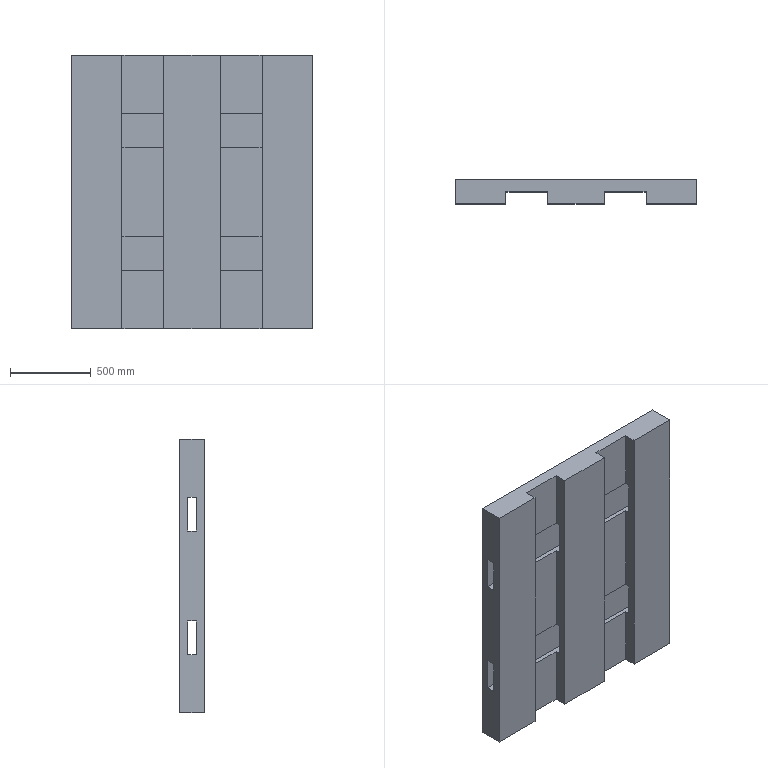Part | STEP file | Tray | 1 solid | 30 faces | box 1500 x 150 x 1700 mm | volume 287460631 mm3 | plane 30
STEP:
#1=CARTESIAN_POINT('',(-750.,-75.,0.));
#2=VERTEX_POINT('',#1);
#3=CARTESIAN_POINT('',(-435.,-75.,0.));
#4=VERTEX_POINT('',#3);
#5=CARTESIAN_POINT('',(-750.,-75.,0.));
#6=DIRECTION('',(1.,0.,0.));
#7=VECTOR('',#6,1000.);
#8=LINE('',#5,#7);
#9=EDGE_CURVE('',#2,#4,#8,.T.);
#10=ORIENTED_EDGE('',*,*,#9,.T.);
#11=CARTESIAN_POINT('',(-435.,-75.,1700.));
#12=VERTEX_POINT('',#11);
#13=CARTESIAN_POINT('',(-435.,-75.,-300.));
#14=DIRECTION('',(0.,0.,1.));
#15=VECTOR('',#14,1000.);
#16=LINE('',#13,#15);
#17=EDGE_CURVE('',#4,#12,#16,.T.);
#18=ORIENTED_EDGE('',*,*,#17,.T.);
#19=CARTESIAN_POINT('',(-750.,-75.,1700.));
#20=VERTEX_POINT('',#19);
#21=CARTESIAN_POINT('',(-750.,-75.,1700.));
#22=DIRECTION('',(1.,0.,0.));
#23=VECTOR('',#22,1000.);
#24=LINE('',#21,#23);
#25=EDGE_CURVE('',#20,#12,#24,.T.);
#26=ORIENTED_EDGE('',*,*,#25,.F.);
#27=CARTESIAN_POINT('',(-750.,-75.,1700.));
#28=DIRECTION('',(0.,0.,-1.));
#29=VECTOR('',#28,1000.);
#30=LINE('',#27,#29);
#31=EDGE_CURVE('',#20,#2,#30,.T.);
#32=ORIENTED_EDGE('',*,*,#31,.T.);
#33=EDGE_LOOP('',(#10,#18,#26,#32));
#34=FACE_OUTER_BOUND('',#33,.T.);
#35=CARTESIAN_POINT('',(-750.,-75.,1700.));
#36=DIRECTION('',(0.,1.,0.));
#37=DIRECTION('',(0.,0.,1.));
#38=AXIS2_PLACEMENT_3D('',#35,#36,#37);
#39=PLANE('',#38);
#40=ADVANCED_FACE('',(#34),#39,.F.);
#41=CARTESIAN_POINT('',(435.,-75.,1700.));
#42=VERTEX_POINT('',#41);
#43=CARTESIAN_POINT('',(750.,-75.,1700.));
#44=VERTEX_POINT('',#43);
#45=CARTESIAN_POINT('',(-750.,-75.,1700.));
#46=DIRECTION('',(1.,0.,0.));
#47=VECTOR('',#46,1000.);
#48=LINE('',#45,#47);
#49=EDGE_CURVE('',#42,#44,#48,.T.);
#50=ORIENTED_EDGE('',*,*,#49,.F.);
#51=CARTESIAN_POINT('',(435.,-75.,0.));
#52=VERTEX_POINT('',#51);
#53=CARTESIAN_POINT('',(435.,-75.,-300.));
#54=DIRECTION('',(0.,0.,1.));
#55=VECTOR('',#54,1000.);
#56=LINE('',#53,#55);
#57=EDGE_CURVE('',#52,#42,#56,.T.);
#58=ORIENTED_EDGE('',*,*,#57,.F.);
#59=CARTESIAN_POINT('',(750.,-75.,0.));
#60=VERTEX_POINT('',#59);
#61=CARTESIAN_POINT('',(-750.,-75.,0.));
#62=DIRECTION('',(1.,0.,0.));
#63=VECTOR('',#62,1000.);
#64=LINE('',#61,#63);
#65=EDGE_CURVE('',#52,#60,#64,.T.);
#66=ORIENTED_EDGE('',*,*,#65,.T.);
#67=CARTESIAN_POINT('',(750.,-75.,1700.));
#68=DIRECTION('',(0.,0.,-1.));
#69=VECTOR('',#68,1000.);
#70=LINE('',#67,#69);
#71=EDGE_CURVE('',#44,#60,#70,.T.);
#72=ORIENTED_EDGE('',*,*,#71,.F.);
#73=EDGE_LOOP('',(#50,#58,#66,#72));
#74=FACE_OUTER_BOUND('',#73,.T.);
#75=CARTESIAN_POINT('',(-750.,-75.,1700.));
#76=DIRECTION('',(0.,1.,0.));
#77=DIRECTION('',(0.,0.,1.));
#78=AXIS2_PLACEMENT_3D('',#75,#76,#77);
#79=PLANE('',#78);
#80=ADVANCED_FACE('',(#74),#79,.F.);
#81=CARTESIAN_POINT('',(-435.,-27.67,1338.848));
#82=VERTEX_POINT('',#81);
#83=CARTESIAN_POINT('',(-750.,-27.67,1338.848));
#84=VERTEX_POINT('',#83);
#85=CARTESIAN_POINT('',(1508.,-27.67,1338.848));
#86=DIRECTION('',(-1.,0.,0.));
#87=VECTOR('',#86,1000.);
#88=LINE('',#85,#87);
#89=EDGE_CURVE('',#82,#84,#88,.T.);
#90=ORIENTED_EDGE('',*,*,#89,.F.);
#91=CARTESIAN_POINT('',(-435.,-27.67,1129.441));
#92=VERTEX_POINT('',#91);
#93=CARTESIAN_POINT('',(-435.,-27.67,1338.848));
#94=DIRECTION('',(0.,0.,-1.));
#95=VECTOR('',#94,1000.);
#96=LINE('',#93,#95);
#97=EDGE_CURVE('',#82,#92,#96,.T.);
#98=ORIENTED_EDGE('',*,*,#97,.T.);
#99=CARTESIAN_POINT('',(-750.,-27.67,1129.441));
#100=VERTEX_POINT('',#99);
#101=CARTESIAN_POINT('',(1508.,-27.67,1129.441));
#102=DIRECTION('',(-1.,0.,0.));
#103=VECTOR('',#102,1000.);
#104=LINE('',#101,#103);
#105=EDGE_CURVE('',#92,#100,#104,.T.);
#106=ORIENTED_EDGE('',*,*,#105,.T.);
#107=CARTESIAN_POINT('',(-750.,-27.67,1338.848));
#108=DIRECTION('',(0.,0.,1.));
#109=VECTOR('',#108,1000.);
#110=LINE('',#107,#109);
#111=EDGE_CURVE('',#100,#84,#110,.T.);
#112=ORIENTED_EDGE('',*,*,#111,.T.);
#113=EDGE_LOOP('',(#90,#98,#106,#112));
#114=FACE_OUTER_BOUND('',#113,.T.);
#115=CARTESIAN_POINT('',(1508.,-27.67,1338.848));
#116=DIRECTION('',(0.,-1.,0.));
#117=DIRECTION('',(0.,0.,-1.));
#118=AXIS2_PLACEMENT_3D('',#115,#116,#117);
#119=PLANE('',#118);
#120=ADVANCED_FACE('',(#114),#119,.F.);
#121=CARTESIAN_POINT('',(750.,-27.67,1129.441));
#122=VERTEX_POINT('',#121);
#123=CARTESIAN_POINT('',(435.,-27.67,1129.441));
#124=VERTEX_POINT('',#123);
#125=CARTESIAN_POINT('',(1508.,-27.67,1129.441));
#126=DIRECTION('',(-1.,0.,0.));
#127=VECTOR('',#126,1000.);
#128=LINE('',#125,#127);
#129=EDGE_CURVE('',#122,#124,#128,.T.);
#130=ORIENTED_EDGE('',*,*,#129,.T.);
#131=CARTESIAN_POINT('',(435.,-27.67,1338.848));
#132=VERTEX_POINT('',#131);
#133=CARTESIAN_POINT('',(435.,-27.67,1338.848));
#134=DIRECTION('',(0.,0.,1.));
#135=VECTOR('',#134,1000.);
#136=LINE('',#133,#135);
#137=EDGE_CURVE('',#124,#132,#136,.T.);
#138=ORIENTED_EDGE('',*,*,#137,.T.);
#139=CARTESIAN_POINT('',(750.,-27.67,1338.848));
#140=VERTEX_POINT('',#139);
#141=CARTESIAN_POINT('',(1508.,-27.67,1338.848));
#142=DIRECTION('',(-1.,0.,0.));
#143=VECTOR('',#142,1000.);
#144=LINE('',#141,#143);
#145=EDGE_CURVE('',#140,#132,#144,.T.);
#146=ORIENTED_EDGE('',*,*,#145,.F.);
#147=CARTESIAN_POINT('',(750.,-27.67,1700.));
#148=DIRECTION('',(0.,0.,1.));
#149=VECTOR('',#148,1000.);
#150=LINE('',#147,#149);
#151=EDGE_CURVE('',#122,#140,#150,.T.);
#152=ORIENTED_EDGE('',*,*,#151,.F.);
#153=EDGE_LOOP('',(#130,#138,#146,#152));
#154=FACE_OUTER_BOUND('',#153,.T.);
#155=CARTESIAN_POINT('',(1508.,-27.67,1338.848));
#156=DIRECTION('',(0.,-1.,0.));
#157=DIRECTION('',(0.,0.,-1.));
#158=AXIS2_PLACEMENT_3D('',#155,#156,#157);
#159=PLANE('',#158);
#160=ADVANCED_FACE('',(#154),#159,.F.);
#161=CARTESIAN_POINT('',(-435.,-27.67,570.559));
#162=VERTEX_POINT('',#161);
#163=CARTESIAN_POINT('',(-750.,-27.67,570.559));
#164=VERTEX_POINT('',#163);
#165=CARTESIAN_POINT('',(1508.,-27.67,570.559));
#166=DIRECTION('',(-1.,0.,0.));
#167=VECTOR('',#166,1000.);
#168=LINE('',#165,#167);
#169=EDGE_CURVE('',#162,#164,#168,.T.);
#170=ORIENTED_EDGE('',*,*,#169,.F.);
#171=CARTESIAN_POINT('',(-435.,-27.67,361.152));
#172=VERTEX_POINT('',#171);
#173=CARTESIAN_POINT('',(-435.,-27.67,361.152));
#174=DIRECTION('',(0.,0.,-1.));
#175=VECTOR('',#174,1000.);
#176=LINE('',#173,#175);
#177=EDGE_CURVE('',#162,#172,#176,.T.);
#178=ORIENTED_EDGE('',*,*,#177,.T.);
#179=CARTESIAN_POINT('',(-750.,-27.67,361.152));
#180=VERTEX_POINT('',#179);
#181=CARTESIAN_POINT('',(1508.,-27.67,361.152));
#182=DIRECTION('',(-1.,0.,0.));
#183=VECTOR('',#182,1000.);
#184=LINE('',#181,#183);
#185=EDGE_CURVE('',#172,#180,#184,.T.);
#186=ORIENTED_EDGE('',*,*,#185,.T.);
#187=CARTESIAN_POINT('',(-750.,-27.67,361.152));
#188=DIRECTION('',(0.,0.,1.));
#189=VECTOR('',#188,1000.);
#190=LINE('',#187,#189);
#191=EDGE_CURVE('',#180,#164,#190,.T.);
#192=ORIENTED_EDGE('',*,*,#191,.T.);
#193=EDGE_LOOP('',(#170,#178,#186,#192));
#194=FACE_OUTER_BOUND('',#193,.T.);
#195=CARTESIAN_POINT('',(1508.,-27.67,361.152));
#196=DIRECTION('',(0.,-1.,0.));
#197=DIRECTION('',(0.,0.,-1.));
#198=AXIS2_PLACEMENT_3D('',#195,#196,#197);
#199=PLANE('',#198);
#200=ADVANCED_FACE('',(#194),#199,.F.);
#201=CARTESIAN_POINT('',(750.,-27.67,361.152));
#202=VERTEX_POINT('',#201);
#203=CARTESIAN_POINT('',(435.,-27.67,361.152));
#204=VERTEX_POINT('',#203);
#205=CARTESIAN_POINT('',(1508.,-27.67,361.152));
#206=DIRECTION('',(-1.,0.,0.));
#207=VECTOR('',#206,1000.);
#208=LINE('',#205,#207);
#209=EDGE_CURVE('',#202,#204,#208,.T.);
#210=ORIENTED_EDGE('',*,*,#209,.T.);
#211=CARTESIAN_POINT('',(435.,-27.67,570.559));
#212=VERTEX_POINT('',#211);
#213=CARTESIAN_POINT('',(435.,-27.67,361.152));
#214=DIRECTION('',(0.,0.,1.));
#215=VECTOR('',#214,1000.);
#216=LINE('',#213,#215);
#217=EDGE_CURVE('',#204,#212,#216,.T.);
#218=ORIENTED_EDGE('',*,*,#217,.T.);
#219=CARTESIAN_POINT('',(750.,-27.67,570.559));
#220=VERTEX_POINT('',#219);
#221=CARTESIAN_POINT('',(1508.,-27.67,570.559));
#222=DIRECTION('',(-1.,0.,0.));
#223=VECTOR('',#222,1000.);
#224=LINE('',#221,#223);
#225=EDGE_CURVE('',#220,#212,#224,.T.);
#226=ORIENTED_EDGE('',*,*,#225,.F.);
#227=CARTESIAN_POINT('',(750.,-27.67,1700.));
#228=DIRECTION('',(0.,0.,1.));
#229=VECTOR('',#228,1000.);
#230=LINE('',#227,#229);
#231=EDGE_CURVE('',#202,#220,#230,.T.);
#232=ORIENTED_EDGE('',*,*,#231,.F.);
#233=EDGE_LOOP('',(#210,#218,#226,#232));
#234=FACE_OUTER_BOUND('',#233,.T.);
#235=CARTESIAN_POINT('',(1508.,-27.67,361.152));
#236=DIRECTION('',(0.,-1.,0.));
#237=DIRECTION('',(0.,0.,-1.));
#238=AXIS2_PLACEMENT_3D('',#235,#236,#237);
#239=PLANE('',#238);
#240=ADVANCED_FACE('',(#234),#239,.F.);
#241=ORIENTED_EDGE('',*,*,#231,.T.);
#242=CARTESIAN_POINT('',(750.,27.67,570.559));
#243=VERTEX_POINT('',#242);
#244=CARTESIAN_POINT('',(750.,75.,570.559));
#245=DIRECTION('',(0.,1.,0.));
#246=VECTOR('',#245,1000.);
#247=LINE('',#244,#246);
#248=EDGE_CURVE('',#220,#243,#247,.T.);
#249=ORIENTED_EDGE('',*,*,#248,.T.);
#250=CARTESIAN_POINT('',(750.,27.67,361.152));
#251=VERTEX_POINT('',#250);
#252=CARTESIAN_POINT('',(750.,27.67,1700.));
#253=DIRECTION('',(0.,0.,-1.));
#254=VECTOR('',#253,1000.);
#255=LINE('',#252,#254);
#256=EDGE_CURVE('',#243,#251,#255,.T.);
#257=ORIENTED_EDGE('',*,*,#256,.T.);
#258=CARTESIAN_POINT('',(750.,75.,361.152));
#259=DIRECTION('',(0.,-1.,0.));
#260=VECTOR('',#259,1000.);
#261=LINE('',#258,#260);
#262=EDGE_CURVE('',#251,#202,#261,.T.);
#263=ORIENTED_EDGE('',*,*,#262,.T.);
#264=EDGE_LOOP('',(#241,#249,#257,#263));
#265=FACE_BOUND('',#264,.T.);
#266=ORIENTED_EDGE('',*,*,#151,.T.);
#267=CARTESIAN_POINT('',(750.,27.67,1338.848));
#268=VERTEX_POINT('',#267);
#269=CARTESIAN_POINT('',(750.,75.,1338.848));
#270=DIRECTION('',(0.,1.,0.));
#271=VECTOR('',#270,1000.);
#272=LINE('',#269,#271);
#273=EDGE_CURVE('',#140,#268,#272,.T.);
#274=ORIENTED_EDGE('',*,*,#273,.T.);
#275=CARTESIAN_POINT('',(750.,27.67,1129.441));
#276=VERTEX_POINT('',#275);
#277=CARTESIAN_POINT('',(750.,27.67,1700.));
#278=DIRECTION('',(0.,0.,-1.));
#279=VECTOR('',#278,1000.);
#280=LINE('',#277,#279);
#281=EDGE_CURVE('',#268,#276,#280,.T.);
#282=ORIENTED_EDGE('',*,*,#281,.T.);
#283=CARTESIAN_POINT('',(750.,75.,1129.441));
#284=DIRECTION('',(0.,-1.,0.));
#285=VECTOR('',#284,1000.);
#286=LINE('',#283,#285);
#287=EDGE_CURVE('',#276,#122,#286,.T.);
#288=ORIENTED_EDGE('',*,*,#287,.T.);
#289=EDGE_LOOP('',(#266,#274,#282,#288));
#290=FACE_BOUND('',#289,.T.);
#291=CARTESIAN_POINT('',(750.,75.,0.));
#292=VERTEX_POINT('',#291);
#293=CARTESIAN_POINT('',(750.,75.,0.));
#294=DIRECTION('',(0.,1.,0.));
#295=VECTOR('',#294,1000.);
#296=LINE('',#293,#295);
#297=EDGE_CURVE('',#60,#292,#296,.T.);
#298=ORIENTED_EDGE('',*,*,#297,.T.);
#299=CARTESIAN_POINT('',(750.,75.,1700.));
#300=VERTEX_POINT('',#299);
#301=CARTESIAN_POINT('',(750.,75.,1700.));
#302=DIRECTION('',(0.,0.,-1.));
#303=VECTOR('',#302,1000.);
#304=LINE('',#301,#303);
#305=EDGE_CURVE('',#300,#292,#304,.T.);
#306=ORIENTED_EDGE('',*,*,#305,.F.);
#307=CARTESIAN_POINT('',(750.,75.,1700.));
#308=DIRECTION('',(0.,1.,0.));
#309=VECTOR('',#308,1000.);
#310=LINE('',#307,#309);
#311=EDGE_CURVE('',#44,#300,#310,.T.);
#312=ORIENTED_EDGE('',*,*,#311,.F.);
#313=ORIENTED_EDGE('',*,*,#71,.T.);
#314=EDGE_LOOP('',(#298,#306,#312,#313));
#315=FACE_OUTER_BOUND('',#314,.T.);
#316=CARTESIAN_POINT('',(750.,75.,1700.));
#317=DIRECTION('',(-1.,0.,0.));
#318=DIRECTION('',(0.,0.,1.));
#319=AXIS2_PLACEMENT_3D('',#316,#317,#318);
#320=PLANE('',#319);
#321=ADVANCED_FACE('',(#265,#290,#315),#320,.F.);
#322=CARTESIAN_POINT('',(-750.,75.,0.));
#323=VERTEX_POINT('',#322);
#324=CARTESIAN_POINT('',(-750.,75.,0.));
#325=DIRECTION('',(-1.,0.,0.));
#326=VECTOR('',#325,1000.);
#327=LINE('',#324,#326);
#328=EDGE_CURVE('',#292,#323,#327,.T.);
#329=ORIENTED_EDGE('',*,*,#328,.T.);
#330=CARTESIAN_POINT('',(-750.,75.,1700.));
#331=VERTEX_POINT('',#330);
#332=CARTESIAN_POINT('',(-750.,75.,1700.));
#333=DIRECTION('',(0.,0.,-1.));
#334=VECTOR('',#333,1000.);
#335=LINE('',#332,#334);
#336=EDGE_CURVE('',#331,#323,#335,.T.);
#337=ORIENTED_EDGE('',*,*,#336,.F.);
#338=CARTESIAN_POINT('',(-750.,75.,1700.));
#339=DIRECTION('',(-1.,0.,0.));
#340=VECTOR('',#339,1000.);
#341=LINE('',#338,#340);
#342=EDGE_CURVE('',#300,#331,#341,.T.);
#343=ORIENTED_EDGE('',*,*,#342,.F.);
#344=ORIENTED_EDGE('',*,*,#305,.T.);
#345=EDGE_LOOP('',(#329,#337,#343,#344));
#346=FACE_OUTER_BOUND('',#345,.T.);
#347=CARTESIAN_POINT('',(-750.,75.,1700.));
#348=DIRECTION('',(0.,-1.,0.));
#349=DIRECTION('',(0.,0.,-1.));
#350=AXIS2_PLACEMENT_3D('',#347,#348,#349);
#351=PLANE('',#350);
#352=ADVANCED_FACE('',(#346),#351,.F.);
#353=CARTESIAN_POINT('',(-750.,27.67,570.559));
#354=VERTEX_POINT('',#353);
#355=CARTESIAN_POINT('',(-750.,27.67,361.152));
#356=VERTEX_POINT('',#355);
#357=CARTESIAN_POINT('',(-750.,27.67,361.152));
#358=DIRECTION('',(0.,0.,-1.));
#359=VECTOR('',#358,1000.);
#360=LINE('',#357,#359);
#361=EDGE_CURVE('',#354,#356,#360,.T.);
#362=ORIENTED_EDGE('',*,*,#361,.F.);
#363=CARTESIAN_POINT('',(-750.,27.67,570.559));
#364=DIRECTION('',(0.,1.,0.));
#365=VECTOR('',#364,1000.);
#366=LINE('',#363,#365);
#367=EDGE_CURVE('',#164,#354,#366,.T.);
#368=ORIENTED_EDGE('',*,*,#367,.F.);
#369=ORIENTED_EDGE('',*,*,#191,.F.);
#370=CARTESIAN_POINT('',(-750.,27.67,361.152));
#371=DIRECTION('',(0.,-1.,0.));
#372=VECTOR('',#371,1000.);
#373=LINE('',#370,#372);
#374=EDGE_CURVE('',#356,#180,#373,.T.);
#375=ORIENTED_EDGE('',*,*,#374,.F.);
#376=EDGE_LOOP('',(#362,#368,#369,#375));
#377=FACE_BOUND('',#376,.T.);
#378=CARTESIAN_POINT('',(-750.,27.67,1338.848));
#379=VERTEX_POINT('',#378);
#380=CARTESIAN_POINT('',(-750.,27.67,1129.441));
#381=VERTEX_POINT('',#380);
#382=CARTESIAN_POINT('',(-750.,27.67,1338.848));
#383=DIRECTION('',(0.,0.,-1.));
#384=VECTOR('',#383,1000.);
#385=LINE('',#382,#384);
#386=EDGE_CURVE('',#379,#381,#385,.T.);
#387=ORIENTED_EDGE('',*,*,#386,.F.);
#388=CARTESIAN_POINT('',(-750.,27.67,1338.848));
#389=DIRECTION('',(0.,1.,0.));
#390=VECTOR('',#389,1000.);
#391=LINE('',#388,#390);
#392=EDGE_CURVE('',#84,#379,#391,.T.);
#393=ORIENTED_EDGE('',*,*,#392,.F.);
#394=ORIENTED_EDGE('',*,*,#111,.F.);
#395=CARTESIAN_POINT('',(-750.,27.67,1129.441));
#396=DIRECTION('',(0.,-1.,0.));
#397=VECTOR('',#396,1000.);
#398=LINE('',#395,#397);
#399=EDGE_CURVE('',#381,#100,#398,.T.);
#400=ORIENTED_EDGE('',*,*,#399,.F.);
#401=EDGE_LOOP('',(#387,#393,#394,#400));
#402=FACE_BOUND('',#401,.T.);
#403=CARTESIAN_POINT('',(-750.,75.,0.));
#404=DIRECTION('',(0.,-1.,0.));
#405=VECTOR('',#404,1000.);
#406=LINE('',#403,#405);
#407=EDGE_CURVE('',#323,#2,#406,.T.);
#408=ORIENTED_EDGE('',*,*,#407,.T.);
#409=ORIENTED_EDGE('',*,*,#31,.F.);
#410=CARTESIAN_POINT('',(-750.,75.,1700.));
#411=DIRECTION('',(0.,-1.,0.));
#412=VECTOR('',#411,1000.);
#413=LINE('',#410,#412);
#414=EDGE_CURVE('',#331,#20,#413,.T.);
#415=ORIENTED_EDGE('',*,*,#414,.F.);
#416=ORIENTED_EDGE('',*,*,#336,.T.);
#417=EDGE_LOOP('',(#408,#409,#415,#416));
#418=FACE_OUTER_BOUND('',#417,.T.);
#419=CARTESIAN_POINT('',(-750.,75.,1700.));
#420=DIRECTION('',(1.,0.,0.));
#421=DIRECTION('',(0.,0.,-1.));
#422=AXIS2_PLACEMENT_3D('',#419,#420,#421);
#423=PLANE('',#422);
#424=ADVANCED_FACE('',(#377,#402,#418),#423,.F.);
#425=CARTESIAN_POINT('',(-175.,-75.,1700.));
#426=VERTEX_POINT('',#425);
#427=CARTESIAN_POINT('',(175.,-75.,1700.));
#428=VERTEX_POINT('',#427);
#429=CARTESIAN_POINT('',(-750.,-75.,1700.));
#430=DIRECTION('',(1.,0.,0.));
#431=VECTOR('',#430,1000.);
#432=LINE('',#429,#431);
#433=EDGE_CURVE('',#426,#428,#432,.T.);
#434=ORIENTED_EDGE('',*,*,#433,.F.);
#435=CARTESIAN_POINT('',(-175.,-75.,0.));
#436=VERTEX_POINT('',#435);
#437=CARTESIAN_POINT('',(-175.,-75.,-300.));
#438=DIRECTION('',(0.,0.,1.));
#439=VECTOR('',#438,1000.);
#440=LINE('',#437,#439);
#441=EDGE_CURVE('',#436,#426,#440,.T.);
#442=ORIENTED_EDGE('',*,*,#441,.F.);
#443=CARTESIAN_POINT('',(175.,-75.,0.));
#444=VERTEX_POINT('',#443);
#445=CARTESIAN_POINT('',(-750.,-75.,0.));
#446=DIRECTION('',(1.,0.,0.));
#447=VECTOR('',#446,1000.);
#448=LINE('',#445,#447);
#449=EDGE_CURVE('',#436,#444,#448,.T.);
#450=ORIENTED_EDGE('',*,*,#449,.T.);
#451=CARTESIAN_POINT('',(175.,-75.,-300.));
#452=DIRECTION('',(0.,0.,1.));
#453=VECTOR('',#452,1000.);
#454=LINE('',#451,#453);
#455=EDGE_CURVE('',#444,#428,#454,.T.);
#456=ORIENTED_EDGE('',*,*,#455,.T.);
#457=EDGE_LOOP('',(#434,#442,#450,#456));
#458=FACE_OUTER_BOUND('',#457,.T.);
#459=CARTESIAN_POINT('',(-750.,-75.,1700.));
#460=DIRECTION('',(0.,1.,0.));
#461=DIRECTION('',(0.,0.,1.));
#462=AXIS2_PLACEMENT_3D('',#459,#460,#461);
#463=PLANE('',#462);
#464=ADVANCED_FACE('',(#458),#463,.F.);
#465=CARTESIAN_POINT('',(-435.,0.,1700.));
#466=VERTEX_POINT('',#465);
#467=CARTESIAN_POINT('',(-435.,-75.,1700.));
#468=DIRECTION('',(0.,-1.,0.));
#469=VECTOR('',#468,1000.);
#470=LINE('',#467,#469);
#471=EDGE_CURVE('',#466,#12,#470,.T.);
#472=ORIENTED_EDGE('',*,*,#471,.F.);
#473=CARTESIAN_POINT('',(-175.,0.,1700.));
#474=VERTEX_POINT('',#473);
#475=CARTESIAN_POINT('',(-435.,0.,1700.));
#476=DIRECTION('',(-1.,0.,0.));
#477=VECTOR('',#476,1000.);
#478=LINE('',#475,#477);
#479=EDGE_CURVE('',#474,#466,#478,.T.);
#480=ORIENTED_EDGE('',*,*,#479,.F.);
#481=CARTESIAN_POINT('',(-175.,0.,1700.));
#482=DIRECTION('',(0.,1.,0.));
#483=VECTOR('',#482,1000.);
#484=LINE('',#481,#483);
#485=EDGE_CURVE('',#426,#474,#484,.T.);
#486=ORIENTED_EDGE('',*,*,#485,.F.);
#487=ORIENTED_EDGE('',*,*,#433,.T.);
#488=CARTESIAN_POINT('',(175.,0.,1700.));
#489=VERTEX_POINT('',#488);
#490=CARTESIAN_POINT('',(175.,0.,1700.));
#491=DIRECTION('',(0.,-1.,0.));
#492=VECTOR('',#491,1000.);
#493=LINE('',#490,#492);
#494=EDGE_CURVE('',#489,#428,#493,.T.);
#495=ORIENTED_EDGE('',*,*,#494,.F.);
#496=CARTESIAN_POINT('',(435.,0.,1700.));
#497=VERTEX_POINT('',#496);
#498=CARTESIAN_POINT('',(435.,0.,1700.));
#499=DIRECTION('',(-1.,0.,0.));
#500=VECTOR('',#499,1000.);
#501=LINE('',#498,#500);
#502=EDGE_CURVE('',#497,#489,#501,.T.);
#503=ORIENTED_EDGE('',*,*,#502,.F.);
#504=CARTESIAN_POINT('',(435.,-75.,1700.));
#505=DIRECTION('',(0.,1.,0.));
#506=VECTOR('',#505,1000.);
#507=LINE('',#504,#506);
#508=EDGE_CURVE('',#42,#497,#507,.T.);
#509=ORIENTED_EDGE('',*,*,#508,.F.);
#510=ORIENTED_EDGE('',*,*,#49,.T.);
#511=ORIENTED_EDGE('',*,*,#311,.T.);
#512=ORIENTED_EDGE('',*,*,#342,.T.);
#513=ORIENTED_EDGE('',*,*,#414,.T.);
#514=ORIENTED_EDGE('',*,*,#25,.T.);
#515=EDGE_LOOP('',(#472,#480,#486,#487,#495,#503,#509,#510,#511,#512,#513,#514));
#516=FACE_OUTER_BOUND('',#515,.T.);
#517=CARTESIAN_POINT('',(0.,0.,1700.));
#518=DIRECTION('',(0.,0.,1.));
#519=DIRECTION('',(1.,0.,0.));
#520=AXIS2_PLACEMENT_3D('',#517,#518,#519);
#521=PLANE('',#520);
#522=ADVANCED_FACE('',(#516),#521,.T.);
#523=CARTESIAN_POINT('',(-175.,0.,0.));
#524=VERTEX_POINT('',#523);
#525=CARTESIAN_POINT('',(-435.,0.,0.));
#526=VERTEX_POINT('',#525);
#527=CARTESIAN_POINT('',(0.,0.,0.));
#528=DIRECTION('',(-1.,0.,0.));
#529=VECTOR('',#528,1000.);
#530=LINE('',#527,#529);
#531=EDGE_CURVE('',#524,#526,#530,.T.);
#532=ORIENTED_EDGE('',*,*,#531,.T.);
#533=CARTESIAN_POINT('',(-435.,0.,0.));
#534=DIRECTION('',(0.,-1.,0.));
#535=VECTOR('',#534,1000.);
#536=LINE('',#533,#535);
#537=EDGE_CURVE('',#526,#4,#536,.T.);
#538=ORIENTED_EDGE('',*,*,#537,.T.);
#539=ORIENTED_EDGE('',*,*,#9,.F.);
#540=ORIENTED_EDGE('',*,*,#407,.F.);
#541=ORIENTED_EDGE('',*,*,#328,.F.);
#542=ORIENTED_EDGE('',*,*,#297,.F.);
#543=ORIENTED_EDGE('',*,*,#65,.F.);
#544=CARTESIAN_POINT('',(435.,0.,0.));
#545=VERTEX_POINT('',#544);
#546=CARTESIAN_POINT('',(435.,0.,0.));
#547=DIRECTION('',(0.,1.,0.));
#548=VECTOR('',#547,1000.);
#549=LINE('',#546,#548);
#550=EDGE_CURVE('',#52,#545,#549,.T.);
#551=ORIENTED_EDGE('',*,*,#550,.T.);
#552=CARTESIAN_POINT('',(175.,0.,0.));
#553=VERTEX_POINT('',#552);
#554=CARTESIAN_POINT('',(0.,0.,0.));
#555=DIRECTION('',(-1.,0.,0.));
#556=VECTOR('',#555,1000.);
#557=LINE('',#554,#556);
#558=EDGE_CURVE('',#545,#553,#557,.T.);
#559=ORIENTED_EDGE('',*,*,#558,.T.);
#560=CARTESIAN_POINT('',(175.,0.,0.));
#561=DIRECTION('',(0.,-1.,0.));
#562=VECTOR('',#561,1000.);
#563=LINE('',#560,#562);
#564=EDGE_CURVE('',#553,#444,#563,.T.);
#565=ORIENTED_EDGE('',*,*,#564,.T.);
#566=ORIENTED_EDGE('',*,*,#449,.F.);
#567=CARTESIAN_POINT('',(-175.,0.,0.));
#568=DIRECTION('',(0.,1.,0.));
#569=VECTOR('',#568,1000.);
#570=LINE('',#567,#569);
#571=EDGE_CURVE('',#436,#524,#570,.T.);
#572=ORIENTED_EDGE('',*,*,#571,.T.);
#573=EDGE_LOOP('',(#532,#538,#539,#540,#541,#542,#543,#551,#559,#565,#566,#572));
#574=FACE_OUTER_BOUND('',#573,.T.);
#575=CARTESIAN_POINT('',(0.,0.,0.));
#576=DIRECTION('',(0.,0.,1.));
#577=DIRECTION('',(1.,0.,0.));
#578=AXIS2_PLACEMENT_3D('',#575,#576,#577);
#579=PLANE('',#578);
#580=ADVANCED_FACE('',(#574),#579,.F.);
#581=CARTESIAN_POINT('',(-175.,0.,1338.848));
#582=VERTEX_POINT('',#581);
#583=CARTESIAN_POINT('',(-435.,0.,1338.848));
#584=VERTEX_POINT('',#583);
#585=CARTESIAN_POINT('',(1508.,0.,1338.848));
#586=DIRECTION('',(-1.,0.,0.));
#587=VECTOR('',#586,1000.);
#588=LINE('',#585,#587);
#589=EDGE_CURVE('',#582,#584,#588,.T.);
#590=ORIENTED_EDGE('',*,*,#589,.T.);
#591=CARTESIAN_POINT('',(-435.,27.67,1338.848));
#592=DIRECTION('',(0.,-1.,0.));
#593=VECTOR('',#592,1000.);
#594=LINE('',#591,#593);
#595=EDGE_CURVE('',#584,#82,#594,.T.);
#596=ORIENTED_EDGE('',*,*,#595,.T.);
#597=ORIENTED_EDGE('',*,*,#89,.T.);
#598=ORIENTED_EDGE('',*,*,#392,.T.);
#599=CARTESIAN_POINT('',(1508.,27.67,1338.848));
#600=DIRECTION('',(-1.,0.,0.));
#601=VECTOR('',#600,1000.);
#602=LINE('',#599,#601);
#603=EDGE_CURVE('',#268,#379,#602,.T.);
#604=ORIENTED_EDGE('',*,*,#603,.F.);
#605=ORIENTED_EDGE('',*,*,#273,.F.);
#606=ORIENTED_EDGE('',*,*,#145,.T.);
#607=CARTESIAN_POINT('',(435.,0.,1338.848));
#608=VERTEX_POINT('',#607);
#609=CARTESIAN_POINT('',(435.,27.67,1338.848));
#610=DIRECTION('',(0.,1.,0.));
#611=VECTOR('',#610,1000.);
#612=LINE('',#609,#611);
#613=EDGE_CURVE('',#132,#608,#612,.T.);
#614=ORIENTED_EDGE('',*,*,#613,.T.);
#615=CARTESIAN_POINT('',(175.,0.,1338.848));
#616=VERTEX_POINT('',#615);
#617=CARTESIAN_POINT('',(1508.,0.,1338.848));
#618=DIRECTION('',(-1.,0.,0.));
#619=VECTOR('',#618,1000.);
#620=LINE('',#617,#619);
#621=EDGE_CURVE('',#608,#616,#620,.T.);
#622=ORIENTED_EDGE('',*,*,#621,.T.);
#623=CARTESIAN_POINT('',(175.,-27.67,1338.848));
#624=VERTEX_POINT('',#623);
#625=CARTESIAN_POINT('',(175.,27.67,1338.848));
#626=DIRECTION('',(0.,-1.,0.));
#627=VECTOR('',#626,1000.);
#628=LINE('',#625,#627);
#629=EDGE_CURVE('',#616,#624,#628,.T.);
#630=ORIENTED_EDGE('',*,*,#629,.T.);
#631=CARTESIAN_POINT('',(-175.,-27.67,1338.848));
#632=VERTEX_POINT('',#631);
#633=CARTESIAN_POINT('',(1508.,-27.67,1338.848));
#634=DIRECTION('',(-1.,0.,0.));
#635=VECTOR('',#634,1000.);
#636=LINE('',#633,#635);
#637=EDGE_CURVE('',#624,#632,#636,.T.);
#638=ORIENTED_EDGE('',*,*,#637,.T.);
#639=CARTESIAN_POINT('',(-175.,27.67,1338.848));
#640=DIRECTION('',(0.,1.,0.));
#641=VECTOR('',#640,1000.);
#642=LINE('',#639,#641);
#643=EDGE_CURVE('',#632,#582,#642,.T.);
#644=ORIENTED_EDGE('',*,*,#643,.T.);
#645=EDGE_LOOP('',(#590,#596,#597,#598,#604,#605,#606,#614,#622,#630,#638,#644));
#646=FACE_OUTER_BOUND('',#645,.T.);
#647=CARTESIAN_POINT('',(1508.,27.67,1338.848));
#648=DIRECTION('',(0.,0.,1.));
#649=DIRECTION('',(1.,0.,0.));
#650=AXIS2_PLACEMENT_3D('',#647,#648,#649);
#651=PLANE('',#650);
#652=ADVANCED_FACE('',(#646),#651,.F.);
#653=CARTESIAN_POINT('',(175.,-27.67,1129.441));
#654=VERTEX_POINT('',#653);
#655=CARTESIAN_POINT('',(-175.,-27.67,1129.441));
#656=VERTEX_POINT('',#655);
#657=CARTESIAN_POINT('',(1508.,-27.67,1129.441));
#658=DIRECTION('',(-1.,0.,0.));
#659=VECTOR('',#658,1000.);
#660=LINE('',#657,#659);
#661=EDGE_CURVE('',#654,#656,#660,.T.);
#662=ORIENTED_EDGE('',*,*,#661,.T.);
#663=CARTESIAN_POINT('',(-175.,-27.67,1338.848));
#664=DIRECTION('',(0.,0.,1.));
#665=VECTOR('',#664,1000.);
#666=LINE('',#663,#665);
#667=EDGE_CURVE('',#656,#632,#666,.T.);
#668=ORIENTED_EDGE('',*,*,#667,.T.);
#669=ORIENTED_EDGE('',*,*,#637,.F.);
#670=CARTESIAN_POINT('',(175.,-27.67,1338.848));
#671=DIRECTION('',(0.,0.,-1.));
#672=VECTOR('',#671,1000.);
#673=LINE('',#670,#672);
#674=EDGE_CURVE('',#624,#654,#673,.T.);
#675=ORIENTED_EDGE('',*,*,#674,.T.);
#676=EDGE_LOOP('',(#662,#668,#669,#675));
#677=FACE_OUTER_BOUND('',#676,.T.);
#678=CARTESIAN_POINT('',(1508.,-27.67,1338.848));
#679=DIRECTION('',(0.,-1.,0.));
#680=DIRECTION('',(0.,0.,-1.));
#681=AXIS2_PLACEMENT_3D('',#678,#679,#680);
#682=PLANE('',#681);
#683=ADVANCED_FACE('',(#677),#682,.F.);
#684=ORIENTED_EDGE('',*,*,#105,.F.);
#685=CARTESIAN_POINT('',(-435.,0.,1129.441));
#686=VERTEX_POINT('',#685);
#687=CARTESIAN_POINT('',(-435.,27.67,1129.441));
#688=DIRECTION('',(0.,1.,0.));
#689=VECTOR('',#688,1000.);
#690=LINE('',#687,#689);
#691=EDGE_CURVE('',#92,#686,#690,.T.);
#692=ORIENTED_EDGE('',*,*,#691,.T.);
#693=CARTESIAN_POINT('',(-175.,0.,1129.441));
#694=VERTEX_POINT('',#693);
#695=CARTESIAN_POINT('',(1508.,0.,1129.441));
#696=DIRECTION('',(1.,0.,0.));
#697=VECTOR('',#696,1000.);
#698=LINE('',#695,#697);
#699=EDGE_CURVE('',#686,#694,#698,.T.);
#700=ORIENTED_EDGE('',*,*,#699,.T.);
#701=CARTESIAN_POINT('',(-175.,27.67,1129.441));
#702=DIRECTION('',(0.,-1.,0.));
#703=VECTOR('',#702,1000.);
#704=LINE('',#701,#703);
#705=EDGE_CURVE('',#694,#656,#704,.T.);
#706=ORIENTED_EDGE('',*,*,#705,.T.);
#707=ORIENTED_EDGE('',*,*,#661,.F.);
#708=CARTESIAN_POINT('',(175.,0.,1129.441));
#709=VERTEX_POINT('',#708);
#710=CARTESIAN_POINT('',(175.,27.67,1129.441));
#711=DIRECTION('',(0.,1.,0.));
#712=VECTOR('',#711,1000.);
#713=LINE('',#710,#712);
#714=EDGE_CURVE('',#654,#709,#713,.T.);
#715=ORIENTED_EDGE('',*,*,#714,.T.);
#716=CARTESIAN_POINT('',(435.,0.,1129.441));
#717=VERTEX_POINT('',#716);
#718=CARTESIAN_POINT('',(1508.,0.,1129.441));
#719=DIRECTION('',(1.,0.,0.));
#720=VECTOR('',#719,1000.);
#721=LINE('',#718,#720);
#722=EDGE_CURVE('',#709,#717,#721,.T.);
#723=ORIENTED_EDGE('',*,*,#722,.T.);
#724=CARTESIAN_POINT('',(435.,27.67,1129.441));
#725=DIRECTION('',(0.,-1.,0.));
#726=VECTOR('',#725,1000.);
#727=LINE('',#724,#726);
#728=EDGE_CURVE('',#717,#124,#727,.T.);
#729=ORIENTED_EDGE('',*,*,#728,.T.);
#730=ORIENTED_EDGE('',*,*,#129,.F.);
#731=ORIENTED_EDGE('',*,*,#287,.F.);
#732=CARTESIAN_POINT('',(1508.,27.67,1129.441));
#733=DIRECTION('',(-1.,0.,0.));
#734=VECTOR('',#733,1000.);
#735=LINE('',#732,#734);
#736=EDGE_CURVE('',#276,#381,#735,.T.);
#737=ORIENTED_EDGE('',*,*,#736,.T.);
#738=ORIENTED_EDGE('',*,*,#399,.T.);
#739=EDGE_LOOP('',(#684,#692,#700,#706,#707,#715,#723,#729,#730,#731,#737,#738));
#740=FACE_OUTER_BOUND('',#739,.T.);
#741=CARTESIAN_POINT('',(1508.,27.67,1129.441));
#742=DIRECTION('',(0.,0.,-1.));
#743=DIRECTION('',(-1.,0.,0.));
#744=AXIS2_PLACEMENT_3D('',#741,#742,#743);
#745=PLANE('',#744);
#746=ADVANCED_FACE('',(#740),#745,.F.);
#747=ORIENTED_EDGE('',*,*,#603,.T.);
#748=ORIENTED_EDGE('',*,*,#386,.T.);
#749=ORIENTED_EDGE('',*,*,#736,.F.);
#750=ORIENTED_EDGE('',*,*,#281,.F.);
#751=EDGE_LOOP('',(#747,#748,#749,#750));
#752=FACE_OUTER_BOUND('',#751,.T.);
#753=CARTESIAN_POINT('',(1508.,27.67,1338.848));
#754=DIRECTION('',(0.,1.,0.));
#755=DIRECTION('',(0.,0.,1.));
#756=AXIS2_PLACEMENT_3D('',#753,#754,#755);
#757=PLANE('',#756);
#758=ADVANCED_FACE('',(#752),#757,.F.);
#759=CARTESIAN_POINT('',(-175.,0.,570.559));
#760=VERTEX_POINT('',#759);
#761=CARTESIAN_POINT('',(-435.,0.,570.559));
#762=VERTEX_POINT('',#761);
#763=CARTESIAN_POINT('',(1508.,0.,570.559));
#764=DIRECTION('',(-1.,0.,0.));
#765=VECTOR('',#764,1000.);
#766=LINE('',#763,#765);
#767=EDGE_CURVE('',#760,#762,#766,.T.);
#768=ORIENTED_EDGE('',*,*,#767,.T.);
#769=CARTESIAN_POINT('',(-435.,27.67,570.559));
#770=DIRECTION('',(0.,-1.,0.));
#771=VECTOR('',#770,1000.);
#772=LINE('',#769,#771);
#773=EDGE_CURVE('',#762,#162,#772,.T.);
#774=ORIENTED_EDGE('',*,*,#773,.T.);
#775=ORIENTED_EDGE('',*,*,#169,.T.);
#776=ORIENTED_EDGE('',*,*,#367,.T.);
#777=CARTESIAN_POINT('',(1508.,27.67,570.559));
#778=DIRECTION('',(-1.,0.,0.));
#779=VECTOR('',#778,1000.);
#780=LINE('',#777,#779);
#781=EDGE_CURVE('',#243,#354,#780,.T.);
#782=ORIENTED_EDGE('',*,*,#781,.F.);
#783=ORIENTED_EDGE('',*,*,#248,.F.);
#784=ORIENTED_EDGE('',*,*,#225,.T.);
#785=CARTESIAN_POINT('',(435.,0.,570.559));
#786=VERTEX_POINT('',#785);
#787=CARTESIAN_POINT('',(435.,27.67,570.559));
#788=DIRECTION('',(0.,1.,0.));
#789=VECTOR('',#788,1000.);
#790=LINE('',#787,#789);
#791=EDGE_CURVE('',#212,#786,#790,.T.);
#792=ORIENTED_EDGE('',*,*,#791,.T.);
#793=CARTESIAN_POINT('',(175.,0.,570.559));
#794=VERTEX_POINT('',#793);
#795=CARTESIAN_POINT('',(1508.,0.,570.559));
#796=DIRECTION('',(-1.,0.,0.));
#797=VECTOR('',#796,1000.);
#798=LINE('',#795,#797);
#799=EDGE_CURVE('',#786,#794,#798,.T.);
#800=ORIENTED_EDGE('',*,*,#799,.T.);
#801=CARTESIAN_POINT('',(175.,-27.67,570.559));
#802=VERTEX_POINT('',#801);
#803=CARTESIAN_POINT('',(175.,27.67,570.559));
#804=DIRECTION('',(0.,-1.,0.));
#805=VECTOR('',#804,1000.);
#806=LINE('',#803,#805);
#807=EDGE_CURVE('',#794,#802,#806,.T.);
#808=ORIENTED_EDGE('',*,*,#807,.T.);
#809=CARTESIAN_POINT('',(-175.,-27.67,570.559));
#810=VERTEX_POINT('',#809);
#811=CARTESIAN_POINT('',(1508.,-27.67,570.559));
#812=DIRECTION('',(-1.,0.,0.));
#813=VECTOR('',#812,1000.);
#814=LINE('',#811,#813);
#815=EDGE_CURVE('',#802,#810,#814,.T.);
#816=ORIENTED_EDGE('',*,*,#815,.T.);
#817=CARTESIAN_POINT('',(-175.,27.67,570.559));
#818=DIRECTION('',(0.,1.,0.));
#819=VECTOR('',#818,1000.);
#820=LINE('',#817,#819);
#821=EDGE_CURVE('',#810,#760,#820,.T.);
#822=ORIENTED_EDGE('',*,*,#821,.T.);
#823=EDGE_LOOP('',(#768,#774,#775,#776,#782,#783,#784,#792,#800,#808,#816,#822));
#824=FACE_OUTER_BOUND('',#823,.T.);
#825=CARTESIAN_POINT('',(1508.,27.67,570.559));
#826=DIRECTION('',(0.,0.,1.));
#827=DIRECTION('',(1.,0.,0.));
#828=AXIS2_PLACEMENT_3D('',#825,#826,#827);
#829=PLANE('',#828);
#830=ADVANCED_FACE('',(#824),#829,.F.);
#831=CARTESIAN_POINT('',(175.,-27.67,361.152));
#832=VERTEX_POINT('',#831);
#833=CARTESIAN_POINT('',(-175.,-27.67,361.152));
#834=VERTEX_POINT('',#833);
#835=CARTESIAN_POINT('',(1508.,-27.67,361.152));
#836=DIRECTION('',(-1.,0.,0.));
#837=VECTOR('',#836,1000.);
#838=LINE('',#835,#837);
#839=EDGE_CURVE('',#832,#834,#838,.T.);
#840=ORIENTED_EDGE('',*,*,#839,.T.);
#841=CARTESIAN_POINT('',(-175.,-27.67,361.152));
#842=DIRECTION('',(0.,0.,1.));
#843=VECTOR('',#842,1000.);
#844=LINE('',#841,#843);
#845=EDGE_CURVE('',#834,#810,#844,.T.);
#846=ORIENTED_EDGE('',*,*,#845,.T.);
#847=ORIENTED_EDGE('',*,*,#815,.F.);
#848=CARTESIAN_POINT('',(175.,-27.67,361.152));
#849=DIRECTION('',(0.,0.,-1.));
#850=VECTOR('',#849,1000.);
#851=LINE('',#848,#850);
#852=EDGE_CURVE('',#802,#832,#851,.T.);
#853=ORIENTED_EDGE('',*,*,#852,.T.);
#854=EDGE_LOOP('',(#840,#846,#847,#853));
#855=FACE_OUTER_BOUND('',#854,.T.);
#856=CARTESIAN_POINT('',(1508.,-27.67,361.152));
#857=DIRECTION('',(0.,-1.,0.));
#858=DIRECTION('',(0.,0.,-1.));
#859=AXIS2_PLACEMENT_3D('',#856,#857,#858);
#860=PLANE('',#859);
#861=ADVANCED_FACE('',(#855),#860,.F.);
#862=ORIENTED_EDGE('',*,*,#185,.F.);
#863=CARTESIAN_POINT('',(-435.,0.,361.152));
#864=VERTEX_POINT('',#863);
#865=CARTESIAN_POINT('',(-435.,27.67,361.152));
#866=DIRECTION('',(0.,1.,0.));
#867=VECTOR('',#866,1000.);
#868=LINE('',#865,#867);
#869=EDGE_CURVE('',#172,#864,#868,.T.);
#870=ORIENTED_EDGE('',*,*,#869,.T.);
#871=CARTESIAN_POINT('',(-175.,0.,361.152));
#872=VERTEX_POINT('',#871);
#873=CARTESIAN_POINT('',(1508.,0.,361.152));
#874=DIRECTION('',(1.,0.,0.));
#875=VECTOR('',#874,1000.);
#876=LINE('',#873,#875);
#877=EDGE_CURVE('',#864,#872,#876,.T.);
#878=ORIENTED_EDGE('',*,*,#877,.T.);
#879=CARTESIAN_POINT('',(-175.,27.67,361.152));
#880=DIRECTION('',(0.,-1.,0.));
#881=VECTOR('',#880,1000.);
#882=LINE('',#879,#881);
#883=EDGE_CURVE('',#872,#834,#882,.T.);
#884=ORIENTED_EDGE('',*,*,#883,.T.);
#885=ORIENTED_EDGE('',*,*,#839,.F.);
#886=CARTESIAN_POINT('',(175.,0.,361.152));
#887=VERTEX_POINT('',#886);
#888=CARTESIAN_POINT('',(175.,27.67,361.152));
#889=DIRECTION('',(0.,1.,0.));
#890=VECTOR('',#889,1000.);
#891=LINE('',#888,#890);
#892=EDGE_CURVE('',#832,#887,#891,.T.);
#893=ORIENTED_EDGE('',*,*,#892,.T.);
#894=CARTESIAN_POINT('',(435.,0.,361.152));
#895=VERTEX_POINT('',#894);
#896=CARTESIAN_POINT('',(1508.,0.,361.152));
#897=DIRECTION('',(1.,0.,0.));
#898=VECTOR('',#897,1000.);
#899=LINE('',#896,#898);
#900=EDGE_CURVE('',#887,#895,#899,.T.);
#901=ORIENTED_EDGE('',*,*,#900,.T.);
#902=CARTESIAN_POINT('',(435.,27.67,361.152));
#903=DIRECTION('',(0.,-1.,0.));
#904=VECTOR('',#903,1000.);
#905=LINE('',#902,#904);
#906=EDGE_CURVE('',#895,#204,#905,.T.);
#907=ORIENTED_EDGE('',*,*,#906,.T.);
#908=ORIENTED_EDGE('',*,*,#209,.F.);
#909=ORIENTED_EDGE('',*,*,#262,.F.);
#910=CARTESIAN_POINT('',(1508.,27.67,361.152));
#911=DIRECTION('',(-1.,0.,0.));
#912=VECTOR('',#911,1000.);
#913=LINE('',#910,#912);
#914=EDGE_CURVE('',#251,#356,#913,.T.);
#915=ORIENTED_EDGE('',*,*,#914,.T.);
#916=ORIENTED_EDGE('',*,*,#374,.T.);
#917=EDGE_LOOP('',(#862,#870,#878,#884,#885,#893,#901,#907,#908,#909,#915,#916));
#918=FACE_OUTER_BOUND('',#917,.T.);
#919=CARTESIAN_POINT('',(1508.,27.67,361.152));
#920=DIRECTION('',(0.,0.,-1.));
#921=DIRECTION('',(-1.,0.,0.));
#922=AXIS2_PLACEMENT_3D('',#919,#920,#921);
#923=PLANE('',#922);
#924=ADVANCED_FACE('',(#918),#923,.F.);
#925=ORIENTED_EDGE('',*,*,#781,.T.);
#926=ORIENTED_EDGE('',*,*,#361,.T.);
#927=ORIENTED_EDGE('',*,*,#914,.F.);
#928=ORIENTED_EDGE('',*,*,#256,.F.);
#929=EDGE_LOOP('',(#925,#926,#927,#928));
#930=FACE_OUTER_BOUND('',#929,.T.);
#931=CARTESIAN_POINT('',(1508.,27.67,361.152));
#932=DIRECTION('',(0.,1.,0.));
#933=DIRECTION('',(0.,0.,1.));
#934=AXIS2_PLACEMENT_3D('',#931,#932,#933);
#935=PLANE('',#934);
#936=ADVANCED_FACE('',(#930),#935,.F.);
#937=CARTESIAN_POINT('',(435.,0.,-300.));
#938=DIRECTION('',(0.,0.,1.));
#939=VECTOR('',#938,1000.);
#940=LINE('',#937,#939);
#941=EDGE_CURVE('',#545,#895,#940,.T.);
#942=ORIENTED_EDGE('',*,*,#941,.T.);
#943=ORIENTED_EDGE('',*,*,#900,.F.);
#944=CARTESIAN_POINT('',(175.,0.,-300.));
#945=DIRECTION('',(0.,0.,1.));
#946=VECTOR('',#945,1000.);
#947=LINE('',#944,#946);
#948=EDGE_CURVE('',#553,#887,#947,.T.);
#949=ORIENTED_EDGE('',*,*,#948,.F.);
#950=ORIENTED_EDGE('',*,*,#558,.F.);
#951=EDGE_LOOP('',(#942,#943,#949,#950));
#952=FACE_OUTER_BOUND('',#951,.T.);
#953=CARTESIAN_POINT('',(435.,0.,-300.));
#954=DIRECTION('',(0.,1.,0.));
#955=DIRECTION('',(-1.,0.,0.));
#956=AXIS2_PLACEMENT_3D('',#953,#954,#955);
#957=PLANE('',#956);
#958=ADVANCED_FACE('',(#952),#957,.F.);
#959=CARTESIAN_POINT('',(435.,0.,-300.));
#960=DIRECTION('',(0.,0.,1.));
#961=VECTOR('',#960,1000.);
#962=LINE('',#959,#961);
#963=EDGE_CURVE('',#608,#497,#962,.T.);
#964=ORIENTED_EDGE('',*,*,#963,.T.);
#965=ORIENTED_EDGE('',*,*,#502,.T.);
#966=CARTESIAN_POINT('',(175.,0.,-300.));
#967=DIRECTION('',(0.,0.,1.));
#968=VECTOR('',#967,1000.);
#969=LINE('',#966,#968);
#970=EDGE_CURVE('',#616,#489,#969,.T.);
#971=ORIENTED_EDGE('',*,*,#970,.F.);
#972=ORIENTED_EDGE('',*,*,#621,.F.);
#973=EDGE_LOOP('',(#964,#965,#971,#972));
#974=FACE_OUTER_BOUND('',#973,.T.);
#975=CARTESIAN_POINT('',(435.,0.,-300.));
#976=DIRECTION('',(0.,1.,0.));
#977=DIRECTION('',(-1.,0.,0.));
#978=AXIS2_PLACEMENT_3D('',#975,#976,#977);
#979=PLANE('',#978);
#980=ADVANCED_FACE('',(#974),#979,.F.);
#981=CARTESIAN_POINT('',(175.,0.,-300.));
#982=DIRECTION('',(0.,0.,1.));
#983=VECTOR('',#982,1000.);
#984=LINE('',#981,#983);
#985=EDGE_CURVE('',#794,#709,#984,.T.);
#986=ORIENTED_EDGE('',*,*,#985,.F.);
#987=ORIENTED_EDGE('',*,*,#799,.F.);
#988=CARTESIAN_POINT('',(435.,0.,-300.));
#989=DIRECTION('',(0.,0.,1.));
#990=VECTOR('',#989,1000.);
#991=LINE('',#988,#990);
#992=EDGE_CURVE('',#786,#717,#991,.T.);
#993=ORIENTED_EDGE('',*,*,#992,.T.);
#994=ORIENTED_EDGE('',*,*,#722,.F.);
#995=EDGE_LOOP('',(#986,#987,#993,#994));
#996=FACE_OUTER_BOUND('',#995,.T.);
#997=CARTESIAN_POINT('',(435.,0.,-300.));
#998=DIRECTION('',(0.,1.,0.));
#999=DIRECTION('',(-1.,0.,0.));
#1000=AXIS2_PLACEMENT_3D('',#997,#998,#999);
#1001=PLANE('',#1000);
#1002=ADVANCED_FACE('',(#996),#1001,.F.);
#1003=ORIENTED_EDGE('',*,*,#57,.T.);
#1004=ORIENTED_EDGE('',*,*,#508,.T.);
#1005=ORIENTED_EDGE('',*,*,#963,.F.);
#1006=ORIENTED_EDGE('',*,*,#613,.F.);
#1007=ORIENTED_EDGE('',*,*,#137,.F.);
#1008=ORIENTED_EDGE('',*,*,#728,.F.);
#1009=ORIENTED_EDGE('',*,*,#992,.F.);
#1010=ORIENTED_EDGE('',*,*,#791,.F.);
#1011=ORIENTED_EDGE('',*,*,#217,.F.);
#1012=ORIENTED_EDGE('',*,*,#906,.F.);
#1013=ORIENTED_EDGE('',*,*,#941,.F.);
#1014=ORIENTED_EDGE('',*,*,#550,.F.);
#1015=EDGE_LOOP('',(#1003,#1004,#1005,#1006,#1007,#1008,#1009,#1010,#1011,#1012,#1013,#1014));
#1016=FACE_OUTER_BOUND('',#1015,.T.);
#1017=CARTESIAN_POINT('',(435.,-75.,-300.));
#1018=DIRECTION('',(1.,0.,0.));
#1019=DIRECTION('',(0.,0.,-1.));
#1020=AXIS2_PLACEMENT_3D('',#1017,#1018,#1019);
#1021=PLANE('',#1020);
#1022=ADVANCED_FACE('',(#1016),#1021,.F.);
#1023=ORIENTED_EDGE('',*,*,#948,.T.);
#1024=ORIENTED_EDGE('',*,*,#892,.F.);
#1025=ORIENTED_EDGE('',*,*,#852,.F.);
#1026=ORIENTED_EDGE('',*,*,#807,.F.);
#1027=ORIENTED_EDGE('',*,*,#985,.T.);
#1028=ORIENTED_EDGE('',*,*,#714,.F.);
#1029=ORIENTED_EDGE('',*,*,#674,.F.);
#1030=ORIENTED_EDGE('',*,*,#629,.F.);
#1031=ORIENTED_EDGE('',*,*,#970,.T.);
#1032=ORIENTED_EDGE('',*,*,#494,.T.);
#1033=ORIENTED_EDGE('',*,*,#455,.F.);
#1034=ORIENTED_EDGE('',*,*,#564,.F.);
#1035=EDGE_LOOP('',(#1023,#1024,#1025,#1026,#1027,#1028,#1029,#1030,#1031,#1032,#1033,#1034));
#1036=FACE_OUTER_BOUND('',#1035,.T.);
#1037=CARTESIAN_POINT('',(175.,0.,-300.));
#1038=DIRECTION('',(-1.,0.,0.));
#1039=DIRECTION('',(0.,-1.,0.));
#1040=AXIS2_PLACEMENT_3D('',#1037,#1038,#1039);
#1041=PLANE('',#1040);
#1042=ADVANCED_FACE('',(#1036),#1041,.F.);
#1043=CARTESIAN_POINT('',(-435.,0.,-300.));
#1044=DIRECTION('',(0.,0.,1.));
#1045=VECTOR('',#1044,1000.);
#1046=LINE('',#1043,#1045);
#1047=EDGE_CURVE('',#526,#864,#1046,.T.);
#1048=ORIENTED_EDGE('',*,*,#1047,.T.);
#1049=ORIENTED_EDGE('',*,*,#869,.F.);
#1050=ORIENTED_EDGE('',*,*,#177,.F.);
#1051=ORIENTED_EDGE('',*,*,#773,.F.);
#1052=CARTESIAN_POINT('',(-435.,0.,-300.));
#1053=DIRECTION('',(0.,0.,1.));
#1054=VECTOR('',#1053,1000.);
#1055=LINE('',#1052,#1054);
#1056=EDGE_CURVE('',#762,#686,#1055,.T.);
#1057=ORIENTED_EDGE('',*,*,#1056,.T.);
#1058=ORIENTED_EDGE('',*,*,#691,.F.);
#1059=ORIENTED_EDGE('',*,*,#97,.F.);
#1060=ORIENTED_EDGE('',*,*,#595,.F.);
#1061=CARTESIAN_POINT('',(-435.,0.,-300.));
#1062=DIRECTION('',(0.,0.,1.));
#1063=VECTOR('',#1062,1000.);
#1064=LINE('',#1061,#1063);
#1065=EDGE_CURVE('',#584,#466,#1064,.T.);
#1066=ORIENTED_EDGE('',*,*,#1065,.T.);
#1067=ORIENTED_EDGE('',*,*,#471,.T.);
#1068=ORIENTED_EDGE('',*,*,#17,.F.);
#1069=ORIENTED_EDGE('',*,*,#537,.F.);
#1070=EDGE_LOOP('',(#1048,#1049,#1050,#1051,#1057,#1058,#1059,#1060,#1066,#1067,#1068,#1069));
#1071=FACE_OUTER_BOUND('',#1070,.T.);
#1072=CARTESIAN_POINT('',(-435.,-75.,-300.));
#1073=DIRECTION('',(-1.,0.,0.));
#1074=DIRECTION('',(0.,0.,1.));
#1075=AXIS2_PLACEMENT_3D('',#1072,#1073,#1074);
#1076=PLANE('',#1075);
#1077=ADVANCED_FACE('',(#1071),#1076,.F.);
#1078=CARTESIAN_POINT('',(-175.,0.,-300.));
#1079=DIRECTION('',(0.,0.,1.));
#1080=VECTOR('',#1079,1000.);
#1081=LINE('',#1078,#1080);
#1082=EDGE_CURVE('',#524,#872,#1081,.T.);
#1083=ORIENTED_EDGE('',*,*,#1082,.T.);
#1084=ORIENTED_EDGE('',*,*,#877,.F.);
#1085=ORIENTED_EDGE('',*,*,#1047,.F.);
#1086=ORIENTED_EDGE('',*,*,#531,.F.);
#1087=EDGE_LOOP('',(#1083,#1084,#1085,#1086));
#1088=FACE_OUTER_BOUND('',#1087,.T.);
#1089=CARTESIAN_POINT('',(-435.,0.,-300.));
#1090=DIRECTION('',(0.,1.,0.));
#1091=DIRECTION('',(0.,0.,1.));
#1092=AXIS2_PLACEMENT_3D('',#1089,#1090,#1091);
#1093=PLANE('',#1092);
#1094=ADVANCED_FACE('',(#1088),#1093,.F.);
#1095=CARTESIAN_POINT('',(-175.,0.,-300.));
#1096=DIRECTION('',(0.,0.,1.));
#1097=VECTOR('',#1096,1000.);
#1098=LINE('',#1095,#1097);
#1099=EDGE_CURVE('',#582,#474,#1098,.T.);
#1100=ORIENTED_EDGE('',*,*,#1099,.T.);
#1101=ORIENTED_EDGE('',*,*,#479,.T.);
#1102=ORIENTED_EDGE('',*,*,#1065,.F.);
#1103=ORIENTED_EDGE('',*,*,#589,.F.);
#1104=EDGE_LOOP('',(#1100,#1101,#1102,#1103));
#1105=FACE_OUTER_BOUND('',#1104,.T.);
#1106=CARTESIAN_POINT('',(-435.,0.,-300.));
#1107=DIRECTION('',(0.,1.,0.));
#1108=DIRECTION('',(0.,0.,1.));
#1109=AXIS2_PLACEMENT_3D('',#1106,#1107,#1108);
#1110=PLANE('',#1109);
#1111=ADVANCED_FACE('',(#1105),#1110,.F.);
#1112=ORIENTED_EDGE('',*,*,#1056,.F.);
#1113=ORIENTED_EDGE('',*,*,#767,.F.);
#1114=CARTESIAN_POINT('',(-175.,0.,-300.));
#1115=DIRECTION('',(0.,0.,1.));
#1116=VECTOR('',#1115,1000.);
#1117=LINE('',#1114,#1116);
#1118=EDGE_CURVE('',#760,#694,#1117,.T.);
#1119=ORIENTED_EDGE('',*,*,#1118,.T.);
#1120=ORIENTED_EDGE('',*,*,#699,.F.);
#1121=EDGE_LOOP('',(#1112,#1113,#1119,#1120));
#1122=FACE_OUTER_BOUND('',#1121,.T.);
#1123=CARTESIAN_POINT('',(-435.,0.,-300.));
#1124=DIRECTION('',(0.,1.,0.));
#1125=DIRECTION('',(0.,0.,1.));
#1126=AXIS2_PLACEMENT_3D('',#1123,#1124,#1125);
#1127=PLANE('',#1126);
#1128=ADVANCED_FACE('',(#1122),#1127,.F.);
#1129=ORIENTED_EDGE('',*,*,#441,.T.);
#1130=ORIENTED_EDGE('',*,*,#485,.T.);
#1131=ORIENTED_EDGE('',*,*,#1099,.F.);
#1132=ORIENTED_EDGE('',*,*,#643,.F.);
#1133=ORIENTED_EDGE('',*,*,#667,.F.);
#1134=ORIENTED_EDGE('',*,*,#705,.F.);
#1135=ORIENTED_EDGE('',*,*,#1118,.F.);
#1136=ORIENTED_EDGE('',*,*,#821,.F.);
#1137=ORIENTED_EDGE('',*,*,#845,.F.);
#1138=ORIENTED_EDGE('',*,*,#883,.F.);
#1139=ORIENTED_EDGE('',*,*,#1082,.F.);
#1140=ORIENTED_EDGE('',*,*,#571,.F.);
#1141=EDGE_LOOP('',(#1129,#1130,#1131,#1132,#1133,#1134,#1135,#1136,#1137,#1138,#1139,#1140));
#1142=FACE_OUTER_BOUND('',#1141,.T.);
#1143=CARTESIAN_POINT('',(-175.,0.,-300.));
#1144=DIRECTION('',(1.,0.,0.));
#1145=DIRECTION('',(0.,1.,0.));
#1146=AXIS2_PLACEMENT_3D('',#1143,#1144,#1145);
#1147=PLANE('',#1146);
#1148=ADVANCED_FACE('',(#1142),#1147,.F.);
#1149=CLOSED_SHELL('',(#40,#80,#120,#160,#200,#240,#321,#352,#424,#464,#522,#580,#652,#683,#746,#758,#830,#861,#924,#936,#958,#980,#1002,#1022,#1042,#1077,#1094,#1111,#1128,#1148));
#1150=MANIFOLD_SOLID_BREP('',#1149);
#1151=CARTESIAN_POINT('',(0.,0.,0.));
#1152=DIRECTION('',(0.,0.,1.));
#1153=DIRECTION('',(1.,0.,0.));
#1154=AXIS2_PLACEMENT_3D('',#1151,#1152,#1153);
#1155=(LENGTH_UNIT()NAMED_UNIT(*)SI_UNIT(.MILLI.,.METRE.));
#1156=UNCERTAINTY_MEASURE_WITH_UNIT(LENGTH_MEASURE(0.00001),#1155,'','');
#1157=(NAMED_UNIT(*)PLANE_ANGLE_UNIT()SI_UNIT($,.RADIAN.));
#1158=(NAMED_UNIT(*)SI_UNIT($,.STERADIAN.)SOLID_ANGLE_UNIT());
#1159=(GEOMETRIC_REPRESENTATION_CONTEXT(3)GLOBAL_UNCERTAINTY_ASSIGNED_CONTEXT((#1156))GLOBAL_UNIT_ASSIGNED_CONTEXT((#1155,#1157,#1158))REPRESENTATION_CONTEXT('',''));
#1160=ADVANCED_BREP_SHAPE_REPRESENTATION('',(#1150,#1154),#1159);